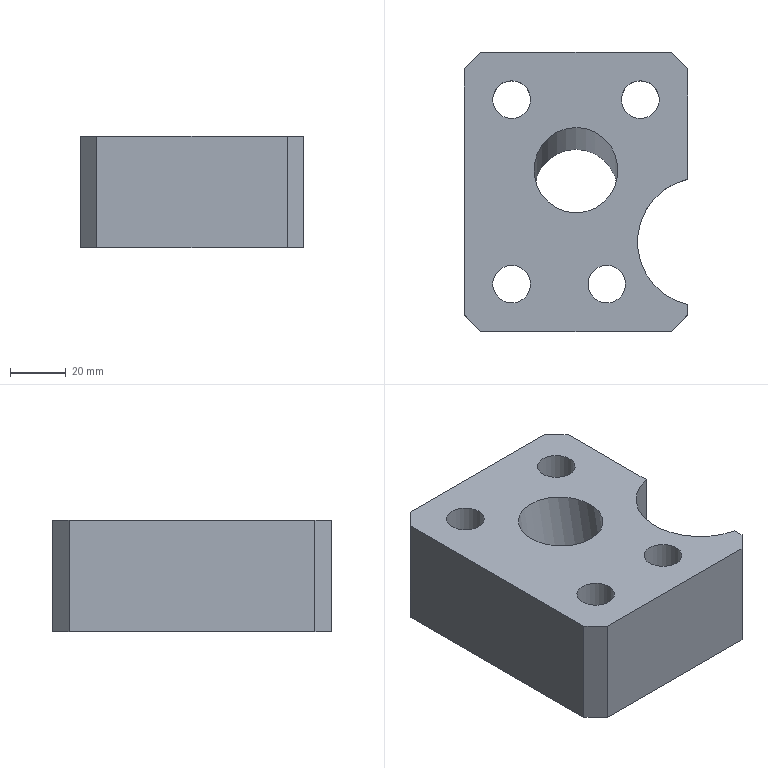Part | STEP file | solid 102 | 1 solid | 25 faces | box 80 x 100 x 40 mm | volume 232410 mm3 | plane 15 | cylinder 10 | commonest cylinder face diameters 13.5 x4 20 x4 30 x1 46 x1